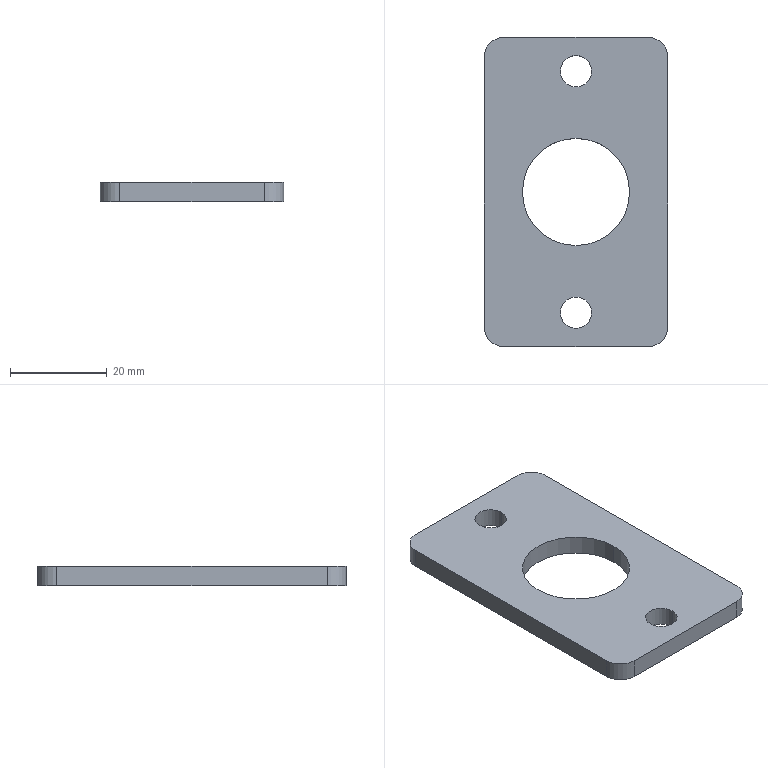Part | STEP file | 04-19 cylinder connection plate | 1 solid | 16 faces | box 38 x 64 x 4 mm | volume 7859 mm3 | cylinder 10 | plane 6 | commonest cylinder face diameters 6.5 x4 8 x4 22.2 x2
STEP:
#1=CARTESIAN_POINT('',(3.25,-25.,0.));
#2=VERTEX_POINT('',#1);
#3=CARTESIAN_POINT('',(-3.25,-25.,0.));
#4=VERTEX_POINT('',#3);
#5=CARTESIAN_POINT('',(0.,-25.,0.));
#6=DIRECTION('',(0.,0.,-1.));
#7=DIRECTION('',(1.,0.,0.));
#8=AXIS2_PLACEMENT_3D('',#5,#6,#7);
#9=CIRCLE('',#8,3.25);
#10=EDGE_CURVE('',#2,#4,#9,.T.);
#11=ORIENTED_EDGE('',*,*,#10,.F.);
#12=CARTESIAN_POINT('',(3.25,-25.,-4.));
#13=VERTEX_POINT('',#12);
#14=CARTESIAN_POINT('',(3.25,-25.,0.));
#15=DIRECTION('',(0.,0.,-1.));
#16=VECTOR('',#15,1000.);
#17=LINE('',#14,#16);
#18=EDGE_CURVE('',#2,#13,#17,.T.);
#19=ORIENTED_EDGE('',*,*,#18,.T.);
#20=CARTESIAN_POINT('',(-3.25,-25.,-4.));
#21=VERTEX_POINT('',#20);
#22=CARTESIAN_POINT('',(0.,-25.,-4.));
#23=DIRECTION('',(0.,0.,-1.));
#24=DIRECTION('',(1.,0.,0.));
#25=AXIS2_PLACEMENT_3D('',#22,#23,#24);
#26=CIRCLE('',#25,3.25);
#27=EDGE_CURVE('',#13,#21,#26,.T.);
#28=ORIENTED_EDGE('',*,*,#27,.T.);
#29=CARTESIAN_POINT('',(-3.25,-25.,0.));
#30=DIRECTION('',(0.,0.,-1.));
#31=VECTOR('',#30,1000.);
#32=LINE('',#29,#31);
#33=EDGE_CURVE('',#4,#21,#32,.T.);
#34=ORIENTED_EDGE('',*,*,#33,.F.);
#35=EDGE_LOOP('',(#11,#19,#28,#34));
#36=FACE_OUTER_BOUND('',#35,.T.);
#37=CARTESIAN_POINT('',(0.,-25.,0.));
#38=DIRECTION('',(0.,0.,-1.));
#39=DIRECTION('',(-1.,0.,0.));
#40=AXIS2_PLACEMENT_3D('',#37,#38,#39);
#41=CYLINDRICAL_SURFACE('',#40,3.25);
#42=ADVANCED_FACE('',(#36),#41,.F.);
#43=CARTESIAN_POINT('',(3.25,25.,0.));
#44=VERTEX_POINT('',#43);
#45=CARTESIAN_POINT('',(-3.25,25.,0.));
#46=VERTEX_POINT('',#45);
#47=CARTESIAN_POINT('',(0.,25.,0.));
#48=DIRECTION('',(0.,0.,-1.));
#49=DIRECTION('',(1.,0.,0.));
#50=AXIS2_PLACEMENT_3D('',#47,#48,#49);
#51=CIRCLE('',#50,3.25);
#52=EDGE_CURVE('',#44,#46,#51,.T.);
#53=ORIENTED_EDGE('',*,*,#52,.F.);
#54=CARTESIAN_POINT('',(3.25,25.,-4.));
#55=VERTEX_POINT('',#54);
#56=CARTESIAN_POINT('',(3.25,25.,0.));
#57=DIRECTION('',(0.,0.,-1.));
#58=VECTOR('',#57,1000.);
#59=LINE('',#56,#58);
#60=EDGE_CURVE('',#44,#55,#59,.T.);
#61=ORIENTED_EDGE('',*,*,#60,.T.);
#62=CARTESIAN_POINT('',(-3.25,25.,-4.));
#63=VERTEX_POINT('',#62);
#64=CARTESIAN_POINT('',(0.,25.,-4.));
#65=DIRECTION('',(0.,0.,-1.));
#66=DIRECTION('',(1.,0.,0.));
#67=AXIS2_PLACEMENT_3D('',#64,#65,#66);
#68=CIRCLE('',#67,3.25);
#69=EDGE_CURVE('',#55,#63,#68,.T.);
#70=ORIENTED_EDGE('',*,*,#69,.T.);
#71=CARTESIAN_POINT('',(-3.25,25.,0.));
#72=DIRECTION('',(0.,0.,-1.));
#73=VECTOR('',#72,1000.);
#74=LINE('',#71,#73);
#75=EDGE_CURVE('',#46,#63,#74,.T.);
#76=ORIENTED_EDGE('',*,*,#75,.F.);
#77=EDGE_LOOP('',(#53,#61,#70,#76));
#78=FACE_OUTER_BOUND('',#77,.T.);
#79=CARTESIAN_POINT('',(0.,25.,0.));
#80=DIRECTION('',(0.,0.,-1.));
#81=DIRECTION('',(-1.,0.,0.));
#82=AXIS2_PLACEMENT_3D('',#79,#80,#81);
#83=CYLINDRICAL_SURFACE('',#82,3.25);
#84=ADVANCED_FACE('',(#78),#83,.F.);
#85=CARTESIAN_POINT('',(11.1,0.,0.));
#86=VERTEX_POINT('',#85);
#87=CARTESIAN_POINT('',(-11.1,0.,0.));
#88=VERTEX_POINT('',#87);
#89=CARTESIAN_POINT('',(0.,0.,0.));
#90=DIRECTION('',(0.,0.,-1.));
#91=DIRECTION('',(1.,0.,0.));
#92=AXIS2_PLACEMENT_3D('',#89,#90,#91);
#93=CIRCLE('',#92,11.1);
#94=EDGE_CURVE('',#86,#88,#93,.T.);
#95=ORIENTED_EDGE('',*,*,#94,.F.);
#96=CARTESIAN_POINT('',(11.1,0.,-4.));
#97=VERTEX_POINT('',#96);
#98=CARTESIAN_POINT('',(11.1,0.,0.));
#99=DIRECTION('',(0.,0.,-1.));
#100=VECTOR('',#99,1000.);
#101=LINE('',#98,#100);
#102=EDGE_CURVE('',#86,#97,#101,.T.);
#103=ORIENTED_EDGE('',*,*,#102,.T.);
#104=CARTESIAN_POINT('',(-11.1,0.,-4.));
#105=VERTEX_POINT('',#104);
#106=CARTESIAN_POINT('',(0.,0.,-4.));
#107=DIRECTION('',(0.,0.,-1.));
#108=DIRECTION('',(1.,0.,0.));
#109=AXIS2_PLACEMENT_3D('',#106,#107,#108);
#110=CIRCLE('',#109,11.1);
#111=EDGE_CURVE('',#97,#105,#110,.T.);
#112=ORIENTED_EDGE('',*,*,#111,.T.);
#113=CARTESIAN_POINT('',(-11.1,0.,0.));
#114=DIRECTION('',(0.,0.,-1.));
#115=VECTOR('',#114,1000.);
#116=LINE('',#113,#115);
#117=EDGE_CURVE('',#88,#105,#116,.T.);
#118=ORIENTED_EDGE('',*,*,#117,.F.);
#119=EDGE_LOOP('',(#95,#103,#112,#118));
#120=FACE_OUTER_BOUND('',#119,.T.);
#121=CARTESIAN_POINT('',(0.,0.,0.));
#122=DIRECTION('',(0.,0.,-1.));
#123=DIRECTION('',(-1.,0.,0.));
#124=AXIS2_PLACEMENT_3D('',#121,#122,#123);
#125=CYLINDRICAL_SURFACE('',#124,11.1);
#126=ADVANCED_FACE('',(#120),#125,.F.);
#127=CARTESIAN_POINT('',(-15.,-32.,-4.));
#128=VERTEX_POINT('',#127);
#129=CARTESIAN_POINT('',(-19.,-28.,-4.));
#130=VERTEX_POINT('',#129);
#131=CARTESIAN_POINT('',(-15.,-28.,-4.));
#132=DIRECTION('',(0.,0.,-1.));
#133=DIRECTION('',(-1.,0.,0.));
#134=AXIS2_PLACEMENT_3D('',#131,#132,#133);
#135=CIRCLE('',#134,4.);
#136=EDGE_CURVE('',#128,#130,#135,.T.);
#137=ORIENTED_EDGE('',*,*,#136,.F.);
#138=CARTESIAN_POINT('',(-15.,-32.,0.));
#139=VERTEX_POINT('',#138);
#140=CARTESIAN_POINT('',(-15.,-32.,0.));
#141=DIRECTION('',(0.,0.,-1.));
#142=VECTOR('',#141,1000.);
#143=LINE('',#140,#142);
#144=EDGE_CURVE('',#139,#128,#143,.T.);
#145=ORIENTED_EDGE('',*,*,#144,.F.);
#146=CARTESIAN_POINT('',(-19.,-28.,0.));
#147=VERTEX_POINT('',#146);
#148=CARTESIAN_POINT('',(-15.,-28.,0.));
#149=DIRECTION('',(0.,0.,-1.));
#150=DIRECTION('',(-1.,0.,0.));
#151=AXIS2_PLACEMENT_3D('',#148,#149,#150);
#152=CIRCLE('',#151,4.);
#153=EDGE_CURVE('',#139,#147,#152,.T.);
#154=ORIENTED_EDGE('',*,*,#153,.T.);
#155=CARTESIAN_POINT('',(-19.,-28.,0.));
#156=DIRECTION('',(0.,0.,-1.));
#157=VECTOR('',#156,1000.);
#158=LINE('',#155,#157);
#159=EDGE_CURVE('',#147,#130,#158,.T.);
#160=ORIENTED_EDGE('',*,*,#159,.T.);
#161=EDGE_LOOP('',(#137,#145,#154,#160));
#162=FACE_OUTER_BOUND('',#161,.T.);
#163=CARTESIAN_POINT('',(-15.,-28.,0.));
#164=DIRECTION('',(0.,0.,-1.));
#165=DIRECTION('',(-1.,0.,0.));
#166=AXIS2_PLACEMENT_3D('',#163,#164,#165);
#167=CYLINDRICAL_SURFACE('',#166,4.);
#168=ADVANCED_FACE('',(#162),#167,.T.);
#169=CARTESIAN_POINT('',(15.,-32.,-4.));
#170=VERTEX_POINT('',#169);
#171=CARTESIAN_POINT('',(15.,-32.,-4.));
#172=DIRECTION('',(-1.,0.,0.));
#173=VECTOR('',#172,1000.);
#174=LINE('',#171,#173);
#175=EDGE_CURVE('',#170,#128,#174,.T.);
#176=ORIENTED_EDGE('',*,*,#175,.F.);
#177=CARTESIAN_POINT('',(15.,-32.,0.));
#178=VERTEX_POINT('',#177);
#179=CARTESIAN_POINT('',(15.,-32.,0.));
#180=DIRECTION('',(0.,0.,-1.));
#181=VECTOR('',#180,1000.);
#182=LINE('',#179,#181);
#183=EDGE_CURVE('',#178,#170,#182,.T.);
#184=ORIENTED_EDGE('',*,*,#183,.F.);
#185=CARTESIAN_POINT('',(15.,-32.,0.));
#186=DIRECTION('',(-1.,0.,0.));
#187=VECTOR('',#186,1000.);
#188=LINE('',#185,#187);
#189=EDGE_CURVE('',#178,#139,#188,.T.);
#190=ORIENTED_EDGE('',*,*,#189,.T.);
#191=ORIENTED_EDGE('',*,*,#144,.T.);
#192=EDGE_LOOP('',(#176,#184,#190,#191));
#193=FACE_OUTER_BOUND('',#192,.T.);
#194=CARTESIAN_POINT('',(15.,-32.,0.));
#195=DIRECTION('',(0.,-1.,0.));
#196=DIRECTION('',(1.,0.,0.));
#197=AXIS2_PLACEMENT_3D('',#194,#195,#196);
#198=PLANE('',#197);
#199=ADVANCED_FACE('',(#193),#198,.T.);
#200=CARTESIAN_POINT('',(19.,-28.,-4.));
#201=VERTEX_POINT('',#200);
#202=CARTESIAN_POINT('',(15.,-28.,-4.));
#203=DIRECTION('',(0.,0.,-1.));
#204=DIRECTION('',(-1.,0.,0.));
#205=AXIS2_PLACEMENT_3D('',#202,#203,#204);
#206=CIRCLE('',#205,4.);
#207=EDGE_CURVE('',#201,#170,#206,.T.);
#208=ORIENTED_EDGE('',*,*,#207,.F.);
#209=CARTESIAN_POINT('',(19.,-28.,0.));
#210=VERTEX_POINT('',#209);
#211=CARTESIAN_POINT('',(19.,-28.,0.));
#212=DIRECTION('',(0.,0.,-1.));
#213=VECTOR('',#212,1000.);
#214=LINE('',#211,#213);
#215=EDGE_CURVE('',#210,#201,#214,.T.);
#216=ORIENTED_EDGE('',*,*,#215,.F.);
#217=CARTESIAN_POINT('',(15.,-28.,0.));
#218=DIRECTION('',(0.,0.,-1.));
#219=DIRECTION('',(-1.,0.,0.));
#220=AXIS2_PLACEMENT_3D('',#217,#218,#219);
#221=CIRCLE('',#220,4.);
#222=EDGE_CURVE('',#210,#178,#221,.T.);
#223=ORIENTED_EDGE('',*,*,#222,.T.);
#224=ORIENTED_EDGE('',*,*,#183,.T.);
#225=EDGE_LOOP('',(#208,#216,#223,#224));
#226=FACE_OUTER_BOUND('',#225,.T.);
#227=CARTESIAN_POINT('',(15.,-28.,0.));
#228=DIRECTION('',(0.,0.,-1.));
#229=DIRECTION('',(-1.,0.,0.));
#230=AXIS2_PLACEMENT_3D('',#227,#228,#229);
#231=CYLINDRICAL_SURFACE('',#230,4.);
#232=ADVANCED_FACE('',(#226),#231,.T.);
#233=CARTESIAN_POINT('',(19.,28.,-4.));
#234=VERTEX_POINT('',#233);
#235=CARTESIAN_POINT('',(19.,28.,-4.));
#236=DIRECTION('',(0.,-1.,0.));
#237=VECTOR('',#236,1000.);
#238=LINE('',#235,#237);
#239=EDGE_CURVE('',#234,#201,#238,.T.);
#240=ORIENTED_EDGE('',*,*,#239,.F.);
#241=CARTESIAN_POINT('',(19.,28.,0.));
#242=VERTEX_POINT('',#241);
#243=CARTESIAN_POINT('',(19.,28.,0.));
#244=DIRECTION('',(0.,0.,-1.));
#245=VECTOR('',#244,1000.);
#246=LINE('',#243,#245);
#247=EDGE_CURVE('',#242,#234,#246,.T.);
#248=ORIENTED_EDGE('',*,*,#247,.F.);
#249=CARTESIAN_POINT('',(19.,28.,0.));
#250=DIRECTION('',(0.,-1.,0.));
#251=VECTOR('',#250,1000.);
#252=LINE('',#249,#251);
#253=EDGE_CURVE('',#242,#210,#252,.T.);
#254=ORIENTED_EDGE('',*,*,#253,.T.);
#255=ORIENTED_EDGE('',*,*,#215,.T.);
#256=EDGE_LOOP('',(#240,#248,#254,#255));
#257=FACE_OUTER_BOUND('',#256,.T.);
#258=CARTESIAN_POINT('',(19.,28.,0.));
#259=DIRECTION('',(1.,0.,0.));
#260=DIRECTION('',(0.,1.,0.));
#261=AXIS2_PLACEMENT_3D('',#258,#259,#260);
#262=PLANE('',#261);
#263=ADVANCED_FACE('',(#257),#262,.T.);
#264=CARTESIAN_POINT('',(15.,32.,-4.));
#265=VERTEX_POINT('',#264);
#266=CARTESIAN_POINT('',(15.,28.,-4.));
#267=DIRECTION('',(0.,0.,-1.));
#268=DIRECTION('',(-1.,0.,0.));
#269=AXIS2_PLACEMENT_3D('',#266,#267,#268);
#270=CIRCLE('',#269,4.);
#271=EDGE_CURVE('',#265,#234,#270,.T.);
#272=ORIENTED_EDGE('',*,*,#271,.F.);
#273=CARTESIAN_POINT('',(15.,32.,0.));
#274=VERTEX_POINT('',#273);
#275=CARTESIAN_POINT('',(15.,32.,0.));
#276=DIRECTION('',(0.,0.,-1.));
#277=VECTOR('',#276,1000.);
#278=LINE('',#275,#277);
#279=EDGE_CURVE('',#274,#265,#278,.T.);
#280=ORIENTED_EDGE('',*,*,#279,.F.);
#281=CARTESIAN_POINT('',(15.,28.,0.));
#282=DIRECTION('',(0.,0.,-1.));
#283=DIRECTION('',(-1.,0.,0.));
#284=AXIS2_PLACEMENT_3D('',#281,#282,#283);
#285=CIRCLE('',#284,4.);
#286=EDGE_CURVE('',#274,#242,#285,.T.);
#287=ORIENTED_EDGE('',*,*,#286,.T.);
#288=ORIENTED_EDGE('',*,*,#247,.T.);
#289=EDGE_LOOP('',(#272,#280,#287,#288));
#290=FACE_OUTER_BOUND('',#289,.T.);
#291=CARTESIAN_POINT('',(15.,28.,0.));
#292=DIRECTION('',(0.,0.,-1.));
#293=DIRECTION('',(-1.,0.,0.));
#294=AXIS2_PLACEMENT_3D('',#291,#292,#293);
#295=CYLINDRICAL_SURFACE('',#294,4.);
#296=ADVANCED_FACE('',(#290),#295,.T.);
#297=CARTESIAN_POINT('',(-15.,32.,-4.));
#298=VERTEX_POINT('',#297);
#299=CARTESIAN_POINT('',(-15.,32.,-4.));
#300=DIRECTION('',(1.,0.,0.));
#301=VECTOR('',#300,1000.);
#302=LINE('',#299,#301);
#303=EDGE_CURVE('',#298,#265,#302,.T.);
#304=ORIENTED_EDGE('',*,*,#303,.F.);
#305=CARTESIAN_POINT('',(-15.,32.,0.));
#306=VERTEX_POINT('',#305);
#307=CARTESIAN_POINT('',(-15.,32.,0.));
#308=DIRECTION('',(0.,0.,-1.));
#309=VECTOR('',#308,1000.);
#310=LINE('',#307,#309);
#311=EDGE_CURVE('',#306,#298,#310,.T.);
#312=ORIENTED_EDGE('',*,*,#311,.F.);
#313=CARTESIAN_POINT('',(-15.,32.,0.));
#314=DIRECTION('',(1.,0.,0.));
#315=VECTOR('',#314,1000.);
#316=LINE('',#313,#315);
#317=EDGE_CURVE('',#306,#274,#316,.T.);
#318=ORIENTED_EDGE('',*,*,#317,.T.);
#319=ORIENTED_EDGE('',*,*,#279,.T.);
#320=EDGE_LOOP('',(#304,#312,#318,#319));
#321=FACE_OUTER_BOUND('',#320,.T.);
#322=CARTESIAN_POINT('',(-15.,32.,0.));
#323=DIRECTION('',(0.,1.,0.));
#324=DIRECTION('',(-1.,0.,0.));
#325=AXIS2_PLACEMENT_3D('',#322,#323,#324);
#326=PLANE('',#325);
#327=ADVANCED_FACE('',(#321),#326,.T.);
#328=CARTESIAN_POINT('',(-19.,28.,-4.));
#329=VERTEX_POINT('',#328);
#330=CARTESIAN_POINT('',(-15.,28.,-4.));
#331=DIRECTION('',(0.,0.,-1.));
#332=DIRECTION('',(-1.,0.,0.));
#333=AXIS2_PLACEMENT_3D('',#330,#331,#332);
#334=CIRCLE('',#333,4.);
#335=EDGE_CURVE('',#329,#298,#334,.T.);
#336=ORIENTED_EDGE('',*,*,#335,.F.);
#337=CARTESIAN_POINT('',(-19.,28.,0.));
#338=VERTEX_POINT('',#337);
#339=CARTESIAN_POINT('',(-19.,28.,0.));
#340=DIRECTION('',(0.,0.,-1.));
#341=VECTOR('',#340,1000.);
#342=LINE('',#339,#341);
#343=EDGE_CURVE('',#338,#329,#342,.T.);
#344=ORIENTED_EDGE('',*,*,#343,.F.);
#345=CARTESIAN_POINT('',(-15.,28.,0.));
#346=DIRECTION('',(0.,0.,-1.));
#347=DIRECTION('',(-1.,0.,0.));
#348=AXIS2_PLACEMENT_3D('',#345,#346,#347);
#349=CIRCLE('',#348,4.);
#350=EDGE_CURVE('',#338,#306,#349,.T.);
#351=ORIENTED_EDGE('',*,*,#350,.T.);
#352=ORIENTED_EDGE('',*,*,#311,.T.);
#353=EDGE_LOOP('',(#336,#344,#351,#352));
#354=FACE_OUTER_BOUND('',#353,.T.);
#355=CARTESIAN_POINT('',(-15.,28.,0.));
#356=DIRECTION('',(0.,0.,-1.));
#357=DIRECTION('',(-1.,0.,0.));
#358=AXIS2_PLACEMENT_3D('',#355,#356,#357);
#359=CYLINDRICAL_SURFACE('',#358,4.);
#360=ADVANCED_FACE('',(#354),#359,.T.);
#361=CARTESIAN_POINT('',(-19.,-28.,-4.));
#362=DIRECTION('',(0.,1.,0.));
#363=VECTOR('',#362,1000.);
#364=LINE('',#361,#363);
#365=EDGE_CURVE('',#130,#329,#364,.T.);
#366=ORIENTED_EDGE('',*,*,#365,.F.);
#367=ORIENTED_EDGE('',*,*,#159,.F.);
#368=CARTESIAN_POINT('',(-19.,-28.,0.));
#369=DIRECTION('',(0.,1.,0.));
#370=VECTOR('',#369,1000.);
#371=LINE('',#368,#370);
#372=EDGE_CURVE('',#147,#338,#371,.T.);
#373=ORIENTED_EDGE('',*,*,#372,.T.);
#374=ORIENTED_EDGE('',*,*,#343,.T.);
#375=EDGE_LOOP('',(#366,#367,#373,#374));
#376=FACE_OUTER_BOUND('',#375,.T.);
#377=CARTESIAN_POINT('',(-19.,-28.,0.));
#378=DIRECTION('',(-1.,0.,0.));
#379=DIRECTION('',(0.,-1.,0.));
#380=AXIS2_PLACEMENT_3D('',#377,#378,#379);
#381=PLANE('',#380);
#382=ADVANCED_FACE('',(#376),#381,.T.);
#383=CARTESIAN_POINT('',(0.,-25.,0.));
#384=DIRECTION('',(0.,0.,-1.));
#385=DIRECTION('',(1.,0.,0.));
#386=AXIS2_PLACEMENT_3D('',#383,#384,#385);
#387=CIRCLE('',#386,3.25);
#388=EDGE_CURVE('',#4,#2,#387,.T.);
#389=ORIENTED_EDGE('',*,*,#388,.T.);
#390=ORIENTED_EDGE('',*,*,#10,.T.);
#391=EDGE_LOOP('',(#389,#390));
#392=FACE_BOUND('',#391,.T.);
#393=CARTESIAN_POINT('',(0.,25.,0.));
#394=DIRECTION('',(0.,0.,-1.));
#395=DIRECTION('',(1.,0.,0.));
#396=AXIS2_PLACEMENT_3D('',#393,#394,#395);
#397=CIRCLE('',#396,3.25);
#398=EDGE_CURVE('',#46,#44,#397,.T.);
#399=ORIENTED_EDGE('',*,*,#398,.T.);
#400=ORIENTED_EDGE('',*,*,#52,.T.);
#401=EDGE_LOOP('',(#399,#400));
#402=FACE_BOUND('',#401,.T.);
#403=CARTESIAN_POINT('',(0.,0.,0.));
#404=DIRECTION('',(0.,0.,-1.));
#405=DIRECTION('',(1.,0.,0.));
#406=AXIS2_PLACEMENT_3D('',#403,#404,#405);
#407=CIRCLE('',#406,11.1);
#408=EDGE_CURVE('',#88,#86,#407,.T.);
#409=ORIENTED_EDGE('',*,*,#408,.T.);
#410=ORIENTED_EDGE('',*,*,#94,.T.);
#411=EDGE_LOOP('',(#409,#410));
#412=FACE_BOUND('',#411,.T.);
#413=ORIENTED_EDGE('',*,*,#153,.F.);
#414=ORIENTED_EDGE('',*,*,#189,.F.);
#415=ORIENTED_EDGE('',*,*,#222,.F.);
#416=ORIENTED_EDGE('',*,*,#253,.F.);
#417=ORIENTED_EDGE('',*,*,#286,.F.);
#418=ORIENTED_EDGE('',*,*,#317,.F.);
#419=ORIENTED_EDGE('',*,*,#350,.F.);
#420=ORIENTED_EDGE('',*,*,#372,.F.);
#421=EDGE_LOOP('',(#413,#414,#415,#416,#417,#418,#419,#420));
#422=FACE_OUTER_BOUND('',#421,.T.);
#423=CARTESIAN_POINT('',(-15.,-28.,0.));
#424=DIRECTION('',(0.,0.,-1.));
#425=DIRECTION('',(-1.,0.,0.));
#426=AXIS2_PLACEMENT_3D('',#423,#424,#425);
#427=PLANE('',#426);
#428=ADVANCED_FACE('',(#392,#402,#412,#422),#427,.F.);
#429=CARTESIAN_POINT('',(0.,-25.,-4.));
#430=DIRECTION('',(0.,0.,-1.));
#431=DIRECTION('',(1.,0.,0.));
#432=AXIS2_PLACEMENT_3D('',#429,#430,#431);
#433=CIRCLE('',#432,3.25);
#434=EDGE_CURVE('',#21,#13,#433,.T.);
#435=ORIENTED_EDGE('',*,*,#434,.F.);
#436=ORIENTED_EDGE('',*,*,#27,.F.);
#437=EDGE_LOOP('',(#435,#436));
#438=FACE_BOUND('',#437,.T.);
#439=CARTESIAN_POINT('',(0.,25.,-4.));
#440=DIRECTION('',(0.,0.,-1.));
#441=DIRECTION('',(1.,0.,0.));
#442=AXIS2_PLACEMENT_3D('',#439,#440,#441);
#443=CIRCLE('',#442,3.25);
#444=EDGE_CURVE('',#63,#55,#443,.T.);
#445=ORIENTED_EDGE('',*,*,#444,.F.);
#446=ORIENTED_EDGE('',*,*,#69,.F.);
#447=EDGE_LOOP('',(#445,#446));
#448=FACE_BOUND('',#447,.T.);
#449=CARTESIAN_POINT('',(0.,0.,-4.));
#450=DIRECTION('',(0.,0.,-1.));
#451=DIRECTION('',(1.,0.,0.));
#452=AXIS2_PLACEMENT_3D('',#449,#450,#451);
#453=CIRCLE('',#452,11.1);
#454=EDGE_CURVE('',#105,#97,#453,.T.);
#455=ORIENTED_EDGE('',*,*,#454,.F.);
#456=ORIENTED_EDGE('',*,*,#111,.F.);
#457=EDGE_LOOP('',(#455,#456));
#458=FACE_BOUND('',#457,.T.);
#459=ORIENTED_EDGE('',*,*,#136,.T.);
#460=ORIENTED_EDGE('',*,*,#365,.T.);
#461=ORIENTED_EDGE('',*,*,#335,.T.);
#462=ORIENTED_EDGE('',*,*,#303,.T.);
#463=ORIENTED_EDGE('',*,*,#271,.T.);
#464=ORIENTED_EDGE('',*,*,#239,.T.);
#465=ORIENTED_EDGE('',*,*,#207,.T.);
#466=ORIENTED_EDGE('',*,*,#175,.T.);
#467=EDGE_LOOP('',(#459,#460,#461,#462,#463,#464,#465,#466));
#468=FACE_OUTER_BOUND('',#467,.T.);
#469=CARTESIAN_POINT('',(-15.,-28.,-4.));
#470=DIRECTION('',(0.,0.,-1.));
#471=DIRECTION('',(-1.,0.,0.));
#472=AXIS2_PLACEMENT_3D('',#469,#470,#471);
#473=PLANE('',#472);
#474=ADVANCED_FACE('',(#438,#448,#458,#468),#473,.T.);
#475=ORIENTED_EDGE('',*,*,#102,.F.);
#476=ORIENTED_EDGE('',*,*,#408,.F.);
#477=ORIENTED_EDGE('',*,*,#117,.T.);
#478=ORIENTED_EDGE('',*,*,#454,.T.);
#479=EDGE_LOOP('',(#475,#476,#477,#478));
#480=FACE_OUTER_BOUND('',#479,.T.);
#481=CARTESIAN_POINT('',(0.,0.,0.));
#482=DIRECTION('',(0.,0.,-1.));
#483=DIRECTION('',(-1.,0.,0.));
#484=AXIS2_PLACEMENT_3D('',#481,#482,#483);
#485=CYLINDRICAL_SURFACE('',#484,11.1);
#486=ADVANCED_FACE('',(#480),#485,.F.);
#487=ORIENTED_EDGE('',*,*,#60,.F.);
#488=ORIENTED_EDGE('',*,*,#398,.F.);
#489=ORIENTED_EDGE('',*,*,#75,.T.);
#490=ORIENTED_EDGE('',*,*,#444,.T.);
#491=EDGE_LOOP('',(#487,#488,#489,#490));
#492=FACE_OUTER_BOUND('',#491,.T.);
#493=CARTESIAN_POINT('',(0.,25.,0.));
#494=DIRECTION('',(0.,0.,-1.));
#495=DIRECTION('',(-1.,0.,0.));
#496=AXIS2_PLACEMENT_3D('',#493,#494,#495);
#497=CYLINDRICAL_SURFACE('',#496,3.25);
#498=ADVANCED_FACE('',(#492),#497,.F.);
#499=ORIENTED_EDGE('',*,*,#18,.F.);
#500=ORIENTED_EDGE('',*,*,#388,.F.);
#501=ORIENTED_EDGE('',*,*,#33,.T.);
#502=ORIENTED_EDGE('',*,*,#434,.T.);
#503=EDGE_LOOP('',(#499,#500,#501,#502));
#504=FACE_OUTER_BOUND('',#503,.T.);
#505=CARTESIAN_POINT('',(0.,-25.,0.));
#506=DIRECTION('',(0.,0.,-1.));
#507=DIRECTION('',(-1.,0.,0.));
#508=AXIS2_PLACEMENT_3D('',#505,#506,#507);
#509=CYLINDRICAL_SURFACE('',#508,3.25);
#510=ADVANCED_FACE('',(#504),#509,.F.);
#511=CLOSED_SHELL('',(#42,#84,#126,#168,#199,#232,#263,#296,#327,#360,#382,#428,#474,#486,#498,#510));
#512=MANIFOLD_SOLID_BREP('',#511);
#513=CARTESIAN_POINT('',(0.,0.,0.));
#514=DIRECTION('',(0.,0.,1.));
#515=DIRECTION('',(1.,0.,0.));
#516=AXIS2_PLACEMENT_3D('',#513,#514,#515);
#517=(LENGTH_UNIT()NAMED_UNIT(*)SI_UNIT(.MILLI.,.METRE.));
#518=UNCERTAINTY_MEASURE_WITH_UNIT(LENGTH_MEASURE(0.00001),#517,'','');
#519=(NAMED_UNIT(*)PLANE_ANGLE_UNIT()SI_UNIT($,.RADIAN.));
#520=(NAMED_UNIT(*)SI_UNIT($,.STERADIAN.)SOLID_ANGLE_UNIT());
#521=(GEOMETRIC_REPRESENTATION_CONTEXT(3)GLOBAL_UNCERTAINTY_ASSIGNED_CONTEXT((#518))GLOBAL_UNIT_ASSIGNED_CONTEXT((#517,#519,#520))REPRESENTATION_CONTEXT('',''));
#522=ADVANCED_BREP_SHAPE_REPRESENTATION('',(#512,#516),#521);